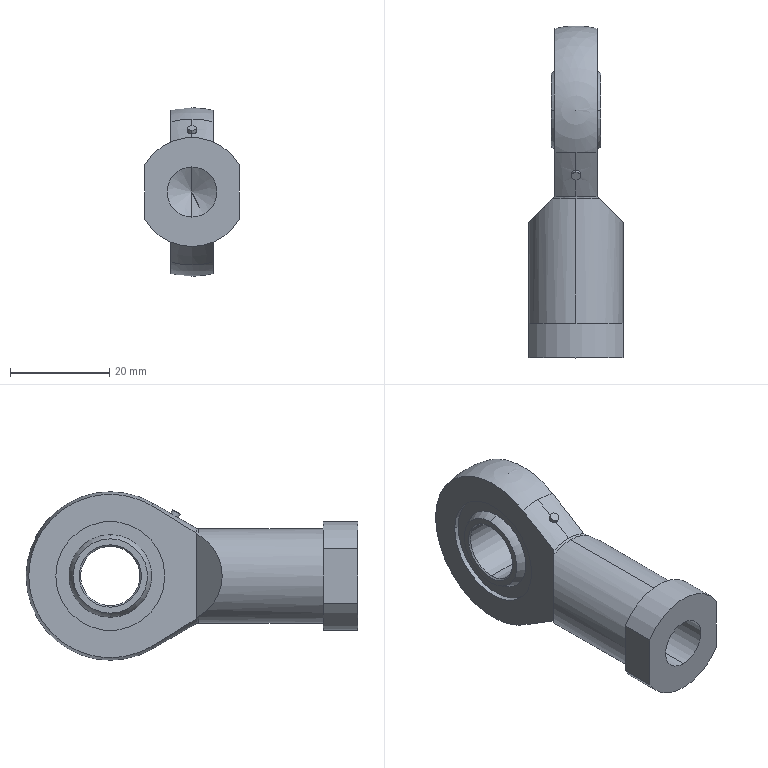Part | SolidWorks | features Revolution 3, ICE 2, RevCut 1 | 1 solid | 47 faces | box 19 x 67 x 34 mm | volume 14399 mm3 | cylinder 15 | plane 14 | cone 9 | torus 7 | sphere 2 | commonest cylinder face diameters 22 x7 1.788 x2 10.106 x2 12 x2 19 x2
STEP:
#1=CARTESIAN_POINT('',(0.,-12.56,13.366));
#2=VERTEX_POINT('',#1);
#3=CARTESIAN_POINT('',(0.,-14.11,12.474));
#4=VERTEX_POINT('',#3);
#5=CARTESIAN_POINT('',(0.,-13.335,12.92));
#6=DIRECTION('',(0.,0.4989,-0.8667));
#7=DIRECTION('',(0.,0.8667,0.4989));
#8=AXIS2_PLACEMENT_3D('',#5,#6,#7);
#9=CIRCLE('',#8,0.8942);
#10=EDGE_CURVE('',#2,#4,#9,.T.);
#11=ORIENTED_EDGE('',*,*,#10,.T.);
#12=CARTESIAN_POINT('',(0.,-13.686,11.737));
#13=VERTEX_POINT('',#12);
#14=CARTESIAN_POINT('',(0.,-13.686,11.737));
#15=DIRECTION('',(0.,0.4989,-0.8667));
#16=VECTOR('',#15,1000.);
#17=LINE('',#14,#16);
#18=EDGE_CURVE('',#4,#13,#17,.T.);
#19=ORIENTED_EDGE('',*,*,#18,.T.);
#20=CARTESIAN_POINT('',(0.,-12.136,12.63));
#21=VERTEX_POINT('',#20);
#22=CARTESIAN_POINT('',(0.,-13.686,11.737));
#23=CARTESIAN_POINT('',(0.1177,-13.686,11.737));
#24=CARTESIAN_POINT('',(0.2343,-13.665,11.748));
#25=CARTESIAN_POINT('',(0.4504,-13.585,11.788));
#26=CARTESIAN_POINT('',(0.5499,-13.525,11.817));
#27=CARTESIAN_POINT('',(0.7147,-13.378,11.893));
#28=CARTESIAN_POINT('',(0.7814,-13.29,11.94));
#29=CARTESIAN_POINT('',(0.8707,-13.101,12.043));
#30=CARTESIAN_POINT('',(0.8942,-12.998,12.1));
#31=CARTESIAN_POINT('',(0.8943,-12.796,12.217));
#32=CARTESIAN_POINT('',(0.8712,-12.696,12.277));
#33=CARTESIAN_POINT('',(0.7813,-12.51,12.39));
#34=CARTESIAN_POINT('',(0.7156,-12.426,12.442));
#35=CARTESIAN_POINT('',(0.5491,-12.286,12.532));
#36=CARTESIAN_POINT('',(0.4502,-12.23,12.568));
#37=CARTESIAN_POINT('',(0.2341,-12.155,12.617));
#38=CARTESIAN_POINT('',(0.1166,-12.136,12.63));
#39=CARTESIAN_POINT('',(0.,-12.136,12.63));
#40=B_SPLINE_CURVE_WITH_KNOTS('',3,(#22,#23,#24,#25,#26,#27,#28,#29,#30,#31,#32,#33,#34,#35,#36,#37,#38,#39),.UNSPECIFIED.,.F.,.F.,(4,2,2,2,2,2,2,2,4),(0.0003219,0.0006715,0.001021,0.001371,0.00172,0.00207,0.002419,0.002769,0.003119),.UNSPECIFIED.);
#41=EDGE_CURVE('',#13,#21,#40,.T.);
#42=ORIENTED_EDGE('',*,*,#41,.T.);
#43=CARTESIAN_POINT('',(0.,-12.136,12.63));
#44=DIRECTION('',(0.,0.4989,-0.8667));
#45=VECTOR('',#44,1000.);
#46=LINE('',#43,#45);
#47=EDGE_CURVE('',#2,#21,#46,.T.);
#48=ORIENTED_EDGE('',*,*,#47,.F.);
#49=EDGE_LOOP('',(#11,#19,#42,#48));
#50=FACE_OUTER_BOUND('',#49,.T.);
#51=CARTESIAN_POINT('',(0.,-12.911,12.183));
#52=DIRECTION('',(0.,0.4989,-0.8667));
#53=DIRECTION('',(0.,0.8667,0.4989));
#54=AXIS2_PLACEMENT_3D('',#51,#52,#53);
#55=CYLINDRICAL_SURFACE('',#54,0.8942);
#56=ADVANCED_FACE('',(#50),#55,.T.);
#57=CARTESIAN_POINT('',(5.,0.,7.5));
#58=VERTEX_POINT('',#57);
#59=CARTESIAN_POINT('',(5.,0.,-7.5));
#60=VERTEX_POINT('',#59);
#61=CARTESIAN_POINT('',(5.,0.,0.));
#62=DIRECTION('',(-1.,0.,0.));
#63=DIRECTION('',(0.,0.,1.));
#64=AXIS2_PLACEMENT_3D('',#61,#62,#63);
#65=CIRCLE('',#64,7.5);
#66=EDGE_CURVE('',#58,#60,#65,.T.);
#67=ORIENTED_EDGE('',*,*,#66,.T.);
#68=CARTESIAN_POINT('',(3.272,0.,-8.353));
#69=VERTEX_POINT('',#68);
#70=CARTESIAN_POINT('',(0.,0.,0.4455));
#71=DIRECTION('',(0.,1.,0.));
#72=DIRECTION('',(0.,0.,1.));
#73=AXIS2_PLACEMENT_3D('',#70,#71,#72);
#74=CIRCLE('',#73,9.388);
#75=EDGE_CURVE('',#60,#69,#74,.T.);
#76=ORIENTED_EDGE('',*,*,#75,.T.);
#77=CARTESIAN_POINT('',(3.272,0.,8.353));
#78=VERTEX_POINT('',#77);
#79=CARTESIAN_POINT('',(3.272,0.,0.));
#80=DIRECTION('',(-1.,0.,0.));
#81=DIRECTION('',(0.,0.,1.));
#82=AXIS2_PLACEMENT_3D('',#79,#80,#81);
#83=CIRCLE('',#82,8.353);
#84=EDGE_CURVE('',#78,#69,#83,.T.);
#85=ORIENTED_EDGE('',*,*,#84,.F.);
#86=CARTESIAN_POINT('',(0.,0.,-0.4455));
#87=DIRECTION('',(0.,-1.,0.));
#88=DIRECTION('',(0.,0.,-1.));
#89=AXIS2_PLACEMENT_3D('',#86,#87,#88);
#90=CIRCLE('',#89,9.388);
#91=EDGE_CURVE('',#58,#78,#90,.T.);
#92=ORIENTED_EDGE('',*,*,#91,.F.);
#93=EDGE_LOOP('',(#67,#76,#85,#92));
#94=FACE_OUTER_BOUND('',#93,.T.);
#95=CARTESIAN_POINT('',(0.,0.,0.));
#96=DIRECTION('',(-1.,0.,0.));
#97=DIRECTION('',(0.,0.,1.));
#98=AXIS2_PLACEMENT_3D('',#95,#96,#97);
#99=TOROIDAL_SURFACE('',#98,-0.4455,9.388);
#100=ADVANCED_FACE('',(#94),#99,.T.);
#101=CARTESIAN_POINT('',(4.7,0.,-6.));
#102=VERTEX_POINT('',#101);
#103=CARTESIAN_POINT('',(4.7,0.,6.));
#104=VERTEX_POINT('',#103);
#105=CARTESIAN_POINT('',(4.7,0.,0.));
#106=DIRECTION('',(-1.,0.,0.));
#107=DIRECTION('',(0.,0.,1.));
#108=AXIS2_PLACEMENT_3D('',#105,#106,#107);
#109=CIRCLE('',#108,6.);
#110=EDGE_CURVE('',#102,#104,#109,.T.);
#111=ORIENTED_EDGE('',*,*,#110,.T.);
#112=CARTESIAN_POINT('',(5.,0.,6.3));
#113=VERTEX_POINT('',#112);
#114=CARTESIAN_POINT('',(4.7,0.,6.));
#115=DIRECTION('',(0.7071,0.,0.7071));
#116=VECTOR('',#115,1000.);
#117=LINE('',#114,#116);
#118=EDGE_CURVE('',#104,#113,#117,.T.);
#119=ORIENTED_EDGE('',*,*,#118,.T.);
#120=CARTESIAN_POINT('',(5.,0.,-6.3));
#121=VERTEX_POINT('',#120);
#122=CARTESIAN_POINT('',(5.,0.,0.));
#123=DIRECTION('',(-1.,0.,0.));
#124=DIRECTION('',(0.,0.,1.));
#125=AXIS2_PLACEMENT_3D('',#122,#123,#124);
#126=CIRCLE('',#125,6.3);
#127=EDGE_CURVE('',#121,#113,#126,.T.);
#128=ORIENTED_EDGE('',*,*,#127,.F.);
#129=CARTESIAN_POINT('',(4.7,0.,-6.));
#130=DIRECTION('',(0.7071,0.,-0.7071));
#131=VECTOR('',#130,1000.);
#132=LINE('',#129,#131);
#133=EDGE_CURVE('',#102,#121,#132,.T.);
#134=ORIENTED_EDGE('',*,*,#133,.F.);
#135=EDGE_LOOP('',(#111,#119,#128,#134));
#136=FACE_OUTER_BOUND('',#135,.T.);
#137=CARTESIAN_POINT('',(4.7,0.,0.));
#138=DIRECTION('',(1.,0.,0.));
#139=DIRECTION('',(0.,0.,-1.));
#140=AXIS2_PLACEMENT_3D('',#137,#138,#139);
#141=CONICAL_SURFACE('',#140,6.,0.7854);
#142=ADVANCED_FACE('',(#136),#141,.F.);
#143=ORIENTED_EDGE('',*,*,#110,.F.);
#144=CARTESIAN_POINT('',(-4.7,0.,-6.));
#145=VERTEX_POINT('',#144);
#146=CARTESIAN_POINT('',(-5.,0.,-6.));
#147=DIRECTION('',(-1.,0.,0.));
#148=VECTOR('',#147,1000.);
#149=LINE('',#146,#148);
#150=EDGE_CURVE('',#102,#145,#149,.T.);
#151=ORIENTED_EDGE('',*,*,#150,.T.);
#152=CARTESIAN_POINT('',(-4.7,0.,6.));
#153=VERTEX_POINT('',#152);
#154=CARTESIAN_POINT('',(-4.7,0.,0.));
#155=DIRECTION('',(-1.,0.,0.));
#156=DIRECTION('',(0.,0.,1.));
#157=AXIS2_PLACEMENT_3D('',#154,#155,#156);
#158=CIRCLE('',#157,6.);
#159=EDGE_CURVE('',#145,#153,#158,.T.);
#160=ORIENTED_EDGE('',*,*,#159,.T.);
#161=CARTESIAN_POINT('',(-5.,0.,6.));
#162=DIRECTION('',(-1.,0.,0.));
#163=VECTOR('',#162,1000.);
#164=LINE('',#161,#163);
#165=EDGE_CURVE('',#104,#153,#164,.T.);
#166=ORIENTED_EDGE('',*,*,#165,.F.);
#167=EDGE_LOOP('',(#143,#151,#160,#166));
#168=FACE_OUTER_BOUND('',#167,.T.);
#169=CARTESIAN_POINT('',(-5.,0.,0.));
#170=DIRECTION('',(-1.,0.,0.));
#171=DIRECTION('',(0.,0.,1.));
#172=AXIS2_PLACEMENT_3D('',#169,#170,#171);
#173=CYLINDRICAL_SURFACE('',#172,6.);
#174=ADVANCED_FACE('',(#168),#173,.F.);
#175=ORIENTED_EDGE('',*,*,#159,.F.);
#176=CARTESIAN_POINT('',(-5.,0.,-6.3));
#177=VERTEX_POINT('',#176);
#178=CARTESIAN_POINT('',(-5.,0.,-6.3));
#179=DIRECTION('',(-0.7071,0.,-0.7071));
#180=VECTOR('',#179,1000.);
#181=LINE('',#178,#180);
#182=EDGE_CURVE('',#145,#177,#181,.T.);
#183=ORIENTED_EDGE('',*,*,#182,.T.);
#184=CARTESIAN_POINT('',(-5.,0.,6.3));
#185=VERTEX_POINT('',#184);
#186=CARTESIAN_POINT('',(-5.,0.,0.));
#187=DIRECTION('',(-1.,0.,0.));
#188=DIRECTION('',(0.,0.,1.));
#189=AXIS2_PLACEMENT_3D('',#186,#187,#188);
#190=CIRCLE('',#189,6.3);
#191=EDGE_CURVE('',#177,#185,#190,.T.);
#192=ORIENTED_EDGE('',*,*,#191,.T.);
#193=CARTESIAN_POINT('',(-5.,0.,6.3));
#194=DIRECTION('',(-0.7071,0.,0.7071));
#195=VECTOR('',#194,1000.);
#196=LINE('',#193,#195);
#197=EDGE_CURVE('',#153,#185,#196,.T.);
#198=ORIENTED_EDGE('',*,*,#197,.F.);
#199=EDGE_LOOP('',(#175,#183,#192,#198));
#200=FACE_OUTER_BOUND('',#199,.T.);
#201=CARTESIAN_POINT('',(-5.,0.,0.));
#202=DIRECTION('',(-1.,0.,0.));
#203=DIRECTION('',(0.,0.,1.));
#204=AXIS2_PLACEMENT_3D('',#201,#202,#203);
#205=CONICAL_SURFACE('',#204,6.3,0.7854);
#206=ADVANCED_FACE('',(#200),#205,.F.);
#207=CARTESIAN_POINT('',(-3.272,0.,8.353));
#208=VERTEX_POINT('',#207);
#209=CARTESIAN_POINT('',(-3.272,0.,-8.353));
#210=VERTEX_POINT('',#209);
#211=CARTESIAN_POINT('',(-3.272,0.,0.));
#212=DIRECTION('',(-1.,0.,0.));
#213=DIRECTION('',(0.,0.,1.));
#214=AXIS2_PLACEMENT_3D('',#211,#212,#213);
#215=CIRCLE('',#214,8.353);
#216=EDGE_CURVE('',#208,#210,#215,.T.);
#217=ORIENTED_EDGE('',*,*,#216,.T.);
#218=CARTESIAN_POINT('',(-5.,0.,-7.5));
#219=VERTEX_POINT('',#218);
#220=CARTESIAN_POINT('',(0.,0.,0.4455));
#221=DIRECTION('',(0.,1.,0.));
#222=DIRECTION('',(0.,0.,1.));
#223=AXIS2_PLACEMENT_3D('',#220,#221,#222);
#224=CIRCLE('',#223,9.388);
#225=EDGE_CURVE('',#210,#219,#224,.T.);
#226=ORIENTED_EDGE('',*,*,#225,.T.);
#227=CARTESIAN_POINT('',(-5.,0.,7.5));
#228=VERTEX_POINT('',#227);
#229=CARTESIAN_POINT('',(-5.,0.,0.));
#230=DIRECTION('',(-1.,0.,0.));
#231=DIRECTION('',(0.,0.,1.));
#232=AXIS2_PLACEMENT_3D('',#229,#230,#231);
#233=CIRCLE('',#232,7.5);
#234=EDGE_CURVE('',#228,#219,#233,.T.);
#235=ORIENTED_EDGE('',*,*,#234,.F.);
#236=CARTESIAN_POINT('',(0.,0.,-0.4455));
#237=DIRECTION('',(0.,-1.,0.));
#238=DIRECTION('',(0.,0.,-1.));
#239=AXIS2_PLACEMENT_3D('',#236,#237,#238);
#240=CIRCLE('',#239,9.388);
#241=EDGE_CURVE('',#208,#228,#240,.T.);
#242=ORIENTED_EDGE('',*,*,#241,.F.);
#243=EDGE_LOOP('',(#217,#226,#235,#242));
#244=FACE_OUTER_BOUND('',#243,.T.);
#245=CARTESIAN_POINT('',(0.,0.,0.));
#246=DIRECTION('',(-1.,0.,0.));
#247=DIRECTION('',(0.,0.,1.));
#248=AXIS2_PLACEMENT_3D('',#245,#246,#247);
#249=TOROIDAL_SURFACE('',#248,-0.4455,9.388);
#250=ADVANCED_FACE('',(#244),#249,.T.);
#251=CARTESIAN_POINT('',(0.,-25.483,0.));
#252=VERTEX_POINT('',#251);
#253=CARTESIAN_POINT('',(0.,-28.4,-5.053));
#254=VERTEX_POINT('',#253);
#255=CARTESIAN_POINT('',(0.,-26.219,-1.275));
#256=DIRECTION('',(0.,-0.5,-0.866));
#257=VECTOR('',#256,1000.);
#258=LINE('',#255,#257);
#259=EDGE_CURVE('',#252,#254,#258,.T.);
#260=ORIENTED_EDGE('',*,*,#259,.F.);
#261=CARTESIAN_POINT('',(0.,-28.4,5.053));
#262=VERTEX_POINT('',#261);
#263=CARTESIAN_POINT('',(0.,-26.219,1.275));
#264=DIRECTION('',(0.,-0.5,0.866));
#265=VECTOR('',#264,1000.);
#266=LINE('',#263,#265);
#267=EDGE_CURVE('',#252,#262,#266,.T.);
#268=ORIENTED_EDGE('',*,*,#267,.T.);
#269=CARTESIAN_POINT('',(0.,-28.4,0.));
#270=DIRECTION('',(0.,1.,0.));
#271=DIRECTION('',(0.,0.,1.));
#272=AXIS2_PLACEMENT_3D('',#269,#270,#271);
#273=CIRCLE('',#272,5.053);
#274=EDGE_CURVE('',#254,#262,#273,.T.);
#275=ORIENTED_EDGE('',*,*,#274,.F.);
#276=EDGE_LOOP('',(#260,#268,#275));
#277=FACE_OUTER_BOUND('',#276,.T.);
#278=CARTESIAN_POINT('',(0.,-26.219,0.));
#279=DIRECTION('',(0.,-1.,0.));
#280=DIRECTION('',(0.,0.,-1.));
#281=AXIS2_PLACEMENT_3D('',#278,#279,#280);
#282=CONICAL_SURFACE('',#281,1.275,1.047);
#283=ADVANCED_FACE('',(#277),#282,.F.);
#284=CARTESIAN_POINT('',(0.,-50.,-5.053));
#285=VERTEX_POINT('',#284);
#286=CARTESIAN_POINT('',(0.,-50.,5.053));
#287=VERTEX_POINT('',#286);
#288=CARTESIAN_POINT('',(0.,-50.,0.));
#289=DIRECTION('',(0.,1.,0.));
#290=DIRECTION('',(0.,0.,1.));
#291=AXIS2_PLACEMENT_3D('',#288,#289,#290);
#292=CIRCLE('',#291,5.053);
#293=EDGE_CURVE('',#285,#287,#292,.T.);
#294=ORIENTED_EDGE('',*,*,#293,.F.);
#295=CARTESIAN_POINT('',(0.,0.,-5.053));
#296=DIRECTION('',(0.,1.,0.));
#297=VECTOR('',#296,1000.);
#298=LINE('',#295,#297);
#299=EDGE_CURVE('',#285,#254,#298,.T.);
#300=ORIENTED_EDGE('',*,*,#299,.T.);
#301=ORIENTED_EDGE('',*,*,#274,.T.);
#302=CARTESIAN_POINT('',(0.,0.,5.053));
#303=DIRECTION('',(0.,1.,0.));
#304=VECTOR('',#303,1000.);
#305=LINE('',#302,#304);
#306=EDGE_CURVE('',#287,#262,#305,.T.);
#307=ORIENTED_EDGE('',*,*,#306,.F.);
#308=EDGE_LOOP('',(#294,#300,#301,#307));
#309=FACE_OUTER_BOUND('',#308,.T.);
#310=CARTESIAN_POINT('',(0.,0.,0.));
#311=DIRECTION('',(0.,1.,0.));
#312=DIRECTION('',(0.,0.,1.));
#313=AXIS2_PLACEMENT_3D('',#310,#311,#312);
#314=CYLINDRICAL_SURFACE('',#313,5.053);
#315=ADVANCED_FACE('',(#309),#314,.F.);
#316=CARTESIAN_POINT('',(0.,-17.84,-9.5));
#317=VERTEX_POINT('',#316);
#318=CARTESIAN_POINT('',(4.749,-17.84,-8.228));
#319=VERTEX_POINT('',#318);
#320=CARTESIAN_POINT('',(0.,-17.84,0.));
#321=DIRECTION('',(0.,-1.,0.));
#322=DIRECTION('',(0.,0.,-1.));
#323=AXIS2_PLACEMENT_3D('',#320,#321,#322);
#324=CIRCLE('',#323,9.5);
#325=EDGE_CURVE('',#317,#319,#324,.T.);
#326=ORIENTED_EDGE('',*,*,#325,.F.);
#327=CARTESIAN_POINT('',(0.,-17.341,-9.633));
#328=VERTEX_POINT('',#327);
#329=CARTESIAN_POINT('',(0.,-17.84,-10.5));
#330=DIRECTION('',(-1.,0.,0.));
#331=DIRECTION('',(0.,0.,1.));
#332=AXIS2_PLACEMENT_3D('',#329,#330,#331);
#333=CIRCLE('',#332,1.);
#334=EDGE_CURVE('',#317,#328,#333,.T.);
#335=ORIENTED_EDGE('',*,*,#334,.T.);
#336=CARTESIAN_POINT('',(4.25,-17.341,-8.645));
#337=VERTEX_POINT('',#336);
#338=CARTESIAN_POINT('',(0.,-17.341,0.));
#339=DIRECTION('',(0.,-1.,0.));
#340=DIRECTION('',(0.,0.,-1.));
#341=AXIS2_PLACEMENT_3D('',#338,#339,#340);
#342=CIRCLE('',#341,9.633);
#343=EDGE_CURVE('',#328,#337,#342,.T.);
#344=ORIENTED_EDGE('',*,*,#343,.T.);
#345=CARTESIAN_POINT('',(4.749,-17.84,-8.228));
#346=CARTESIAN_POINT('',(4.568,-17.659,-8.332));
#347=CARTESIAN_POINT('',(4.402,-17.493,-8.473));
#348=CARTESIAN_POINT('',(4.25,-17.341,-8.645));
#349=B_SPLINE_CURVE_WITH_KNOTS('',3,(#345,#346,#347,#348),.UNSPECIFIED.,.F.,.F.,(4,4),(0.000000302,0.00082),.UNSPECIFIED.);
#350=EDGE_CURVE('',#319,#337,#349,.T.);
#351=ORIENTED_EDGE('',*,*,#350,.F.);
#352=EDGE_LOOP('',(#326,#335,#344,#351));
#353=FACE_OUTER_BOUND('',#352,.T.);
#354=CARTESIAN_POINT('',(0.,-17.84,0.));
#355=DIRECTION('',(0.,-1.,0.));
#356=DIRECTION('',(0.,0.,-1.));
#357=AXIS2_PLACEMENT_3D('',#354,#355,#356);
#358=TOROIDAL_SURFACE('',#357,10.5,1.);
#359=ADVANCED_FACE('',(#353),#358,.F.);
#360=CARTESIAN_POINT('',(4.749,-17.84,8.228));
#361=VERTEX_POINT('',#360);
#362=CARTESIAN_POINT('',(0.,-17.84,9.5));
#363=VERTEX_POINT('',#362);
#364=CARTESIAN_POINT('',(0.,-17.84,0.));
#365=DIRECTION('',(0.,-1.,0.));
#366=DIRECTION('',(0.,0.,-1.));
#367=AXIS2_PLACEMENT_3D('',#364,#365,#366);
#368=CIRCLE('',#367,9.5);
#369=EDGE_CURVE('',#361,#363,#368,.T.);
#370=ORIENTED_EDGE('',*,*,#369,.T.);
#371=CARTESIAN_POINT('',(0.,-43.,9.5));
#372=VERTEX_POINT('',#371);
#373=CARTESIAN_POINT('',(0.,-50.,9.5));
#374=DIRECTION('',(0.,-1.,0.));
#375=VECTOR('',#374,1000.);
#376=LINE('',#373,#375);
#377=EDGE_CURVE('',#363,#372,#376,.T.);
#378=ORIENTED_EDGE('',*,*,#377,.T.);
#379=CARTESIAN_POINT('',(9.5,-43.,0.));
#380=VERTEX_POINT('',#379);
#381=CARTESIAN_POINT('',(0.,-43.,0.));
#382=DIRECTION('',(0.,-1.,0.));
#383=DIRECTION('',(0.,0.,-1.));
#384=AXIS2_PLACEMENT_3D('',#381,#382,#383);
#385=CIRCLE('',#384,9.5);
#386=EDGE_CURVE('',#380,#372,#385,.T.);
#387=ORIENTED_EDGE('',*,*,#386,.F.);
#388=CARTESIAN_POINT('',(0.,-43.,-9.5));
#389=VERTEX_POINT('',#388);
#390=CARTESIAN_POINT('',(0.,-43.,0.));
#391=DIRECTION('',(0.,-1.,0.));
#392=DIRECTION('',(0.,0.,-1.));
#393=AXIS2_PLACEMENT_3D('',#390,#391,#392);
#394=CIRCLE('',#393,9.5);
#395=EDGE_CURVE('',#389,#380,#394,.T.);
#396=ORIENTED_EDGE('',*,*,#395,.F.);
#397=CARTESIAN_POINT('',(0.,-50.,-9.5));
#398=DIRECTION('',(0.,-1.,0.));
#399=VECTOR('',#398,1000.);
#400=LINE('',#397,#399);
#401=EDGE_CURVE('',#317,#389,#400,.T.);
#402=ORIENTED_EDGE('',*,*,#401,.F.);
#403=ORIENTED_EDGE('',*,*,#325,.T.);
#404=CARTESIAN_POINT('',(4.749,-17.84,8.228));
#405=CARTESIAN_POINT('',(11.876,-24.967,4.114));
#406=CARTESIAN_POINT('',(11.876,-24.967,-4.114));
#407=CARTESIAN_POINT('',(4.749,-17.84,-8.228));
#408=(BOUNDED_CURVE()B_SPLINE_CURVE(3,(#404,#405,#406,#407),.UNSPECIFIED.,.F.,.T.)B_SPLINE_CURVE_WITH_KNOTS((4,4),(5.236,7.331),.UNSPECIFIED.)CURVE()GEOMETRIC_REPRESENTATION_ITEM()RATIONAL_B_SPLINE_CURVE((1.,0.6666,0.6666,1.))REPRESENTATION_ITEM(''));
#409=EDGE_CURVE('',#361,#319,#408,.T.);
#410=ORIENTED_EDGE('',*,*,#409,.F.);
#411=EDGE_LOOP('',(#370,#378,#387,#396,#402,#403,#410));
#412=FACE_OUTER_BOUND('',#411,.T.);
#413=CARTESIAN_POINT('',(0.,-50.,0.));
#414=DIRECTION('',(0.,-1.,0.));
#415=DIRECTION('',(0.,0.,-1.));
#416=AXIS2_PLACEMENT_3D('',#413,#414,#415);
#417=CYLINDRICAL_SURFACE('',#416,9.5);
#418=ADVANCED_FACE('',(#412),#417,.T.);
#419=CARTESIAN_POINT('',(0.,17.,0.));
#420=VERTEX_POINT('',#419);
#421=CARTESIAN_POINT('',(4.25,16.46,0.));
#422=VERTEX_POINT('',#421);
#423=CARTESIAN_POINT('',(0.,0.,0.));
#424=DIRECTION('',(0.,0.,-1.));
#425=DIRECTION('',(-1.,0.,0.));
#426=AXIS2_PLACEMENT_3D('',#423,#424,#425);
#427=CIRCLE('',#426,17.);
#428=EDGE_CURVE('',#420,#422,#427,.T.);
#429=ORIENTED_EDGE('',*,*,#428,.F.);
#430=CARTESIAN_POINT('',(-4.25,16.46,0.));
#431=VERTEX_POINT('',#430);
#432=CARTESIAN_POINT('',(0.,0.,0.));
#433=DIRECTION('',(0.,0.,1.));
#434=DIRECTION('',(1.,0.,0.));
#435=AXIS2_PLACEMENT_3D('',#432,#433,#434);
#436=CIRCLE('',#435,17.);
#437=EDGE_CURVE('',#420,#431,#436,.T.);
#438=ORIENTED_EDGE('',*,*,#437,.T.);
#439=CARTESIAN_POINT('',(-4.25,-8.481,14.107));
#440=VERTEX_POINT('',#439);
#441=CARTESIAN_POINT('',(-4.25,0.,0.));
#442=DIRECTION('',(-1.,0.,0.));
#443=DIRECTION('',(0.,1.,0.));
#444=AXIS2_PLACEMENT_3D('',#441,#442,#443);
#445=CIRCLE('',#444,16.46);
#446=EDGE_CURVE('',#440,#431,#445,.T.);
#447=ORIENTED_EDGE('',*,*,#446,.F.);
#448=CARTESIAN_POINT('',(0.,-8.481,14.733));
#449=VERTEX_POINT('',#448);
#450=CARTESIAN_POINT('',(0.,-8.481,0.));
#451=DIRECTION('',(0.,-1.,0.));
#452=DIRECTION('',(0.,0.,-1.));
#453=AXIS2_PLACEMENT_3D('',#450,#451,#452);
#454=CIRCLE('',#453,14.733);
#455=EDGE_CURVE('',#449,#440,#454,.T.);
#456=ORIENTED_EDGE('',*,*,#455,.F.);
#457=CARTESIAN_POINT('',(4.25,-8.481,14.107));
#458=VERTEX_POINT('',#457);
#459=CARTESIAN_POINT('',(0.,-8.481,0.));
#460=DIRECTION('',(0.,-1.,0.));
#461=DIRECTION('',(0.,0.,-1.));
#462=AXIS2_PLACEMENT_3D('',#459,#460,#461);
#463=CIRCLE('',#462,14.733);
#464=EDGE_CURVE('',#458,#449,#463,.T.);
#465=ORIENTED_EDGE('',*,*,#464,.F.);
#466=CARTESIAN_POINT('',(4.25,0.,0.));
#467=DIRECTION('',(1.,0.,0.));
#468=DIRECTION('',(0.,-1.,0.));
#469=AXIS2_PLACEMENT_3D('',#466,#467,#468);
#470=CIRCLE('',#469,16.46);
#471=EDGE_CURVE('',#422,#458,#470,.T.);
#472=ORIENTED_EDGE('',*,*,#471,.F.);
#473=EDGE_LOOP('',(#429,#438,#447,#456,#465,#472));
#474=FACE_OUTER_BOUND('',#473,.T.);
#475=CARTESIAN_POINT('',(0.,0.,0.));
#476=DIRECTION('',(0.,0.,1.));
#477=DIRECTION('',(1.,0.,0.));
#478=AXIS2_PLACEMENT_3D('',#475,#476,#477);
#479=SPHERICAL_SURFACE('',#478,17.);
#480=ADVANCED_FACE('',(#474),#479,.T.);
#481=CARTESIAN_POINT('',(0.,-17.341,9.633));
#482=VERTEX_POINT('',#481);
#483=CARTESIAN_POINT('',(-4.25,-17.341,8.645));
#484=VERTEX_POINT('',#483);
#485=CARTESIAN_POINT('',(0.,-17.341,0.));
#486=DIRECTION('',(0.,-1.,0.));
#487=DIRECTION('',(0.,0.,-1.));
#488=AXIS2_PLACEMENT_3D('',#485,#486,#487);
#489=CIRCLE('',#488,9.633);
#490=EDGE_CURVE('',#482,#484,#489,.T.);
#491=ORIENTED_EDGE('',*,*,#490,.F.);
#492=CARTESIAN_POINT('',(0.,-17.341,9.633));
#493=DIRECTION('',(0.,0.8667,0.4989));
#494=VECTOR('',#493,1000.);
#495=LINE('',#492,#494);
#496=EDGE_CURVE('',#482,#13,#495,.T.);
#497=ORIENTED_EDGE('',*,*,#496,.T.);
#498=CARTESIAN_POINT('',(0.,-12.136,12.63));
#499=CARTESIAN_POINT('',(-0.1166,-12.136,12.63));
#500=CARTESIAN_POINT('',(-0.2343,-12.156,12.617));
#501=CARTESIAN_POINT('',(-0.4496,-12.23,12.568));
#502=CARTESIAN_POINT('',(-0.5492,-12.286,12.531));
#503=CARTESIAN_POINT('',(-0.7145,-12.425,12.443));
#504=CARTESIAN_POINT('',(-0.7808,-12.509,12.39));
#505=CARTESIAN_POINT('',(-0.8709,-12.694,12.277));
#506=CARTESIAN_POINT('',(-0.8942,-12.794,12.218));
#507=CARTESIAN_POINT('',(-0.8943,-12.998,12.1));
#508=CARTESIAN_POINT('',(-0.8711,-13.1,12.043));
#509=CARTESIAN_POINT('',(-0.7816,-13.29,11.94));
#510=CARTESIAN_POINT('',(-0.7152,-13.378,11.893));
#511=CARTESIAN_POINT('',(-0.5506,-13.525,11.818));
#512=CARTESIAN_POINT('',(-0.4513,-13.584,11.788));
#513=CARTESIAN_POINT('',(-0.2337,-13.665,11.747));
#514=CARTESIAN_POINT('',(-0.1177,-13.686,11.737));
#515=CARTESIAN_POINT('',(0.,-13.686,11.737));
#516=B_SPLINE_CURVE_WITH_KNOTS('',3,(#498,#499,#500,#501,#502,#503,#504,#505,#506,#507,#508,#509,#510,#511,#512,#513,#514,#515),.UNSPECIFIED.,.F.,.F.,(4,2,2,2,2,2,2,2,4),(0.003119,0.003468,0.003818,0.004167,0.004517,0.004866,0.005215,0.005565,0.005914),.UNSPECIFIED.);
#517=EDGE_CURVE('',#21,#13,#516,.T.);
#518=ORIENTED_EDGE('',*,*,#517,.F.);
#519=CARTESIAN_POINT('',(0.,-17.341,9.633));
#520=DIRECTION('',(0.,0.8667,0.4989));
#521=VECTOR('',#520,1000.);
#522=LINE('',#519,#521);
#523=EDGE_CURVE('',#21,#449,#522,.T.);
#524=ORIENTED_EDGE('',*,*,#523,.T.);
#525=ORIENTED_EDGE('',*,*,#455,.T.);
#526=CARTESIAN_POINT('',(-4.25,-17.341,8.645));
#527=CARTESIAN_POINT('',(-4.25,-15.882,9.581));
#528=CARTESIAN_POINT('',(-4.25,-14.409,10.498));
#529=CARTESIAN_POINT('',(-4.25,-11.452,12.314));
#530=CARTESIAN_POINT('',(-4.25,-9.968,13.213));
#531=CARTESIAN_POINT('',(-4.25,-8.481,14.107));
#532=B_SPLINE_CURVE_WITH_KNOTS('',3,(#526,#527,#528,#529,#530,#531),.UNSPECIFIED.,.F.,.F.,(4,2,4),(0.05787,0.06306,0.06824),.UNSPECIFIED.);
#533=EDGE_CURVE('',#484,#440,#532,.T.);
#534=ORIENTED_EDGE('',*,*,#533,.F.);
#535=EDGE_LOOP('',(#491,#497,#518,#524,#525,#534));
#536=FACE_OUTER_BOUND('',#535,.T.);
#537=CARTESIAN_POINT('',(0.,-17.341,0.));
#538=DIRECTION('',(0.,1.,0.));
#539=DIRECTION('',(0.,0.,1.));
#540=AXIS2_PLACEMENT_3D('',#537,#538,#539);
#541=CONICAL_SURFACE('',#540,9.633,0.5223);
#542=ADVANCED_FACE('',(#536),#541,.T.);
#543=CARTESIAN_POINT('',(-9.5,-43.,-5.545));
#544=VERTEX_POINT('',#543);
#545=CARTESIAN_POINT('',(0.,-43.,-11.));
#546=VERTEX_POINT('',#545);
#547=CARTESIAN_POINT('',(0.,-43.,0.));
#548=DIRECTION('',(0.,-1.,0.));
#549=DIRECTION('',(0.,0.,-1.));
#550=AXIS2_PLACEMENT_3D('',#547,#548,#549);
#551=CIRCLE('',#550,11.);
#552=EDGE_CURVE('',#544,#546,#551,.T.);
#553=ORIENTED_EDGE('',*,*,#552,.T.);
#554=CARTESIAN_POINT('',(0.,-50.,-11.));
#555=VERTEX_POINT('',#554);
#556=CARTESIAN_POINT('',(0.,-50.,-11.));
#557=DIRECTION('',(0.,-1.,0.));
#558=VECTOR('',#557,1000.);
#559=LINE('',#556,#558);
#560=EDGE_CURVE('',#546,#555,#559,.T.);
#561=ORIENTED_EDGE('',*,*,#560,.T.);
#562=CARTESIAN_POINT('',(-9.5,-50.,-5.545));
#563=VERTEX_POINT('',#562);
#564=CARTESIAN_POINT('',(0.,-50.,0.));
#565=DIRECTION('',(0.,-1.,0.));
#566=DIRECTION('',(0.,0.,-1.));
#567=AXIS2_PLACEMENT_3D('',#564,#565,#566);
#568=CIRCLE('',#567,11.);
#569=EDGE_CURVE('',#563,#555,#568,.T.);
#570=ORIENTED_EDGE('',*,*,#569,.F.);
#571=CARTESIAN_POINT('',(-9.5,-50.,-5.545));
#572=DIRECTION('',(0.,-1.,0.));
#573=VECTOR('',#572,1000.);
#574=LINE('',#571,#573);
#575=EDGE_CURVE('',#544,#563,#574,.T.);
#576=ORIENTED_EDGE('',*,*,#575,.F.);
#577=EDGE_LOOP('',(#553,#561,#570,#576));
#578=FACE_OUTER_BOUND('',#577,.T.);
#579=CARTESIAN_POINT('',(0.,-50.,0.));
#580=DIRECTION('',(0.,-1.,0.));
#581=DIRECTION('',(0.,0.,-1.));
#582=AXIS2_PLACEMENT_3D('',#579,#580,#581);
#583=CYLINDRICAL_SURFACE('',#582,11.);
#584=ADVANCED_FACE('',(#578),#583,.T.);
#585=CARTESIAN_POINT('',(-4.25,11.,0.));
#586=VERTEX_POINT('',#585);
#587=CARTESIAN_POINT('',(-4.25,-11.,0.));
#588=VERTEX_POINT('',#587);
#589=CARTESIAN_POINT('',(-4.25,0.,0.));
#590=DIRECTION('',(-1.,0.,0.));
#591=DIRECTION('',(0.,1.,0.));
#592=AXIS2_PLACEMENT_3D('',#589,#590,#591);
#593=CIRCLE('',#592,11.);
#594=EDGE_CURVE('',#586,#588,#593,.T.);
#595=ORIENTED_EDGE('',*,*,#594,.T.);
#596=CARTESIAN_POINT('',(-3.272,-11.,0.));
#597=VERTEX_POINT('',#596);
#598=CARTESIAN_POINT('',(-9.5,-11.,0.));
#599=DIRECTION('',(1.,0.,0.));
#600=VECTOR('',#599,1000.);
#601=LINE('',#598,#600);
#602=EDGE_CURVE('',#588,#597,#601,.T.);
#603=ORIENTED_EDGE('',*,*,#602,.T.);
#604=CARTESIAN_POINT('',(-3.272,11.,0.));
#605=VERTEX_POINT('',#604);
#606=CARTESIAN_POINT('',(-3.272,0.,0.));
#607=DIRECTION('',(-1.,0.,0.));
#608=DIRECTION('',(0.,0.,1.));
#609=AXIS2_PLACEMENT_3D('',#606,#607,#608);
#610=CIRCLE('',#609,11.);
#611=EDGE_CURVE('',#605,#597,#610,.T.);
#612=ORIENTED_EDGE('',*,*,#611,.F.);
#613=CARTESIAN_POINT('',(-9.5,11.,0.));
#614=DIRECTION('',(1.,0.,0.));
#615=VECTOR('',#614,1000.);
#616=LINE('',#613,#615);
#617=EDGE_CURVE('',#586,#605,#616,.T.);
#618=ORIENTED_EDGE('',*,*,#617,.F.);
#619=EDGE_LOOP('',(#595,#603,#612,#618));
#620=FACE_OUTER_BOUND('',#619,.T.);
#621=CARTESIAN_POINT('',(-9.5,0.,0.));
#622=DIRECTION('',(1.,0.,0.));
#623=DIRECTION('',(0.,1.,0.));
#624=AXIS2_PLACEMENT_3D('',#621,#622,#623);
#625=CYLINDRICAL_SURFACE('',#624,11.);
#626=ADVANCED_FACE('',(#620),#625,.F.);
#627=CARTESIAN_POINT('',(3.272,11.,0.));
#628=VERTEX_POINT('',#627);
#629=CARTESIAN_POINT('',(3.272,-11.,0.));
#630=VERTEX_POINT('',#629);
#631=CARTESIAN_POINT('',(3.272,0.,0.));
#632=DIRECTION('',(-1.,0.,0.));
#633=DIRECTION('',(0.,0.,1.));
#634=AXIS2_PLACEMENT_3D('',#631,#632,#633);
#635=CIRCLE('',#634,11.);
#636=EDGE_CURVE('',#628,#630,#635,.T.);
#637=ORIENTED_EDGE('',*,*,#636,.T.);
#638=CARTESIAN_POINT('',(4.25,-11.,0.));
#639=VERTEX_POINT('',#638);
#640=CARTESIAN_POINT('',(-9.5,-11.,0.));
#641=DIRECTION('',(1.,0.,0.));
#642=VECTOR('',#641,1000.);
#643=LINE('',#640,#642);
#644=EDGE_CURVE('',#630,#639,#643,.T.);
#645=ORIENTED_EDGE('',*,*,#644,.T.);
#646=CARTESIAN_POINT('',(4.25,11.,0.));
#647=VERTEX_POINT('',#646);
#648=CARTESIAN_POINT('',(4.25,0.,0.));
#649=DIRECTION('',(-1.,0.,0.));
#650=DIRECTION('',(0.,-1.,0.));
#651=AXIS2_PLACEMENT_3D('',#648,#649,#650);
#652=CIRCLE('',#651,11.);
#653=EDGE_CURVE('',#647,#639,#652,.T.);
#654=ORIENTED_EDGE('',*,*,#653,.F.);
#655=CARTESIAN_POINT('',(-9.5,11.,0.));
#656=DIRECTION('',(1.,0.,0.));
#657=VECTOR('',#656,1000.);
#658=LINE('',#655,#657);
#659=EDGE_CURVE('',#628,#647,#658,.T.);
#660=ORIENTED_EDGE('',*,*,#659,.F.);
#661=EDGE_LOOP('',(#637,#645,#654,#660));
#662=FACE_OUTER_BOUND('',#661,.T.);
#663=CARTESIAN_POINT('',(-9.5,0.,0.));
#664=DIRECTION('',(1.,0.,0.));
#665=DIRECTION('',(0.,1.,0.));
#666=AXIS2_PLACEMENT_3D('',#663,#664,#665);
#667=CYLINDRICAL_SURFACE('',#666,11.);
#668=ADVANCED_FACE('',(#662),#667,.F.);
#669=ORIENTED_EDGE('',*,*,#644,.F.);
#670=CARTESIAN_POINT('',(3.272,0.,0.));
#671=DIRECTION('',(-1.,0.,0.));
#672=DIRECTION('',(0.,0.,1.));
#673=AXIS2_PLACEMENT_3D('',#670,#671,#672);
#674=CIRCLE('',#673,11.);
#675=EDGE_CURVE('',#630,#628,#674,.T.);
#676=ORIENTED_EDGE('',*,*,#675,.T.);
#677=ORIENTED_EDGE('',*,*,#659,.T.);
#678=CARTESIAN_POINT('',(4.25,0.,0.));
#679=DIRECTION('',(-1.,0.,0.));
#680=DIRECTION('',(0.,-1.,0.));
#681=AXIS2_PLACEMENT_3D('',#678,#679,#680);
#682=CIRCLE('',#681,11.);
#683=EDGE_CURVE('',#639,#647,#682,.T.);
#684=ORIENTED_EDGE('',*,*,#683,.F.);
#685=EDGE_LOOP('',(#669,#676,#677,#684));
#686=FACE_OUTER_BOUND('',#685,.T.);
#687=CARTESIAN_POINT('',(-9.5,0.,0.));
#688=DIRECTION('',(1.,0.,0.));
#689=DIRECTION('',(0.,1.,0.));
#690=AXIS2_PLACEMENT_3D('',#687,#688,#689);
#691=CYLINDRICAL_SURFACE('',#690,11.);
#692=ADVANCED_FACE('',(#686),#691,.F.);
#693=ORIENTED_EDGE('',*,*,#602,.F.);
#694=CARTESIAN_POINT('',(-4.25,0.,0.));
#695=DIRECTION('',(-1.,0.,0.));
#696=DIRECTION('',(0.,1.,0.));
#697=AXIS2_PLACEMENT_3D('',#694,#695,#696);
#698=CIRCLE('',#697,11.);
#699=EDGE_CURVE('',#588,#586,#698,.T.);
#700=ORIENTED_EDGE('',*,*,#699,.T.);
#701=ORIENTED_EDGE('',*,*,#617,.T.);
#702=CARTESIAN_POINT('',(-3.272,0.,0.));
#703=DIRECTION('',(-1.,0.,0.));
#704=DIRECTION('',(0.,0.,1.));
#705=AXIS2_PLACEMENT_3D('',#702,#703,#704);
#706=CIRCLE('',#705,11.);
#707=EDGE_CURVE('',#597,#605,#706,.T.);
#708=ORIENTED_EDGE('',*,*,#707,.F.);
#709=EDGE_LOOP('',(#693,#700,#701,#708));
#710=FACE_OUTER_BOUND('',#709,.T.);
#711=CARTESIAN_POINT('',(-9.5,0.,0.));
#712=DIRECTION('',(1.,0.,0.));
#713=DIRECTION('',(0.,1.,0.));
#714=AXIS2_PLACEMENT_3D('',#711,#712,#713);
#715=CYLINDRICAL_SURFACE('',#714,11.);
#716=ADVANCED_FACE('',(#710),#715,.F.);
#717=CARTESIAN_POINT('',(4.25,-17.341,8.645));
#718=VERTEX_POINT('',#717);
#719=CARTESIAN_POINT('',(4.25,-8.481,14.107));
#720=CARTESIAN_POINT('',(4.25,-9.968,13.213));
#721=CARTESIAN_POINT('',(4.25,-11.451,12.315));
#722=CARTESIAN_POINT('',(4.25,-14.408,10.499));
#723=CARTESIAN_POINT('',(4.25,-15.88,9.582));
#724=CARTESIAN_POINT('',(4.25,-17.341,8.645));
#725=B_SPLINE_CURVE_WITH_KNOTS('',3,(#719,#720,#721,#722,#723,#724),.UNSPECIFIED.,.F.,.F.,(4,2,4),(0.02144,0.02664,0.03184),.UNSPECIFIED.);
#726=EDGE_CURVE('',#458,#718,#725,.T.);
#727=ORIENTED_EDGE('',*,*,#726,.T.);
#728=CARTESIAN_POINT('',(4.25,-17.341,-17.));
#729=DIRECTION('',(0.,0.,1.));
#730=VECTOR('',#729,1000.);
#731=LINE('',#728,#730);
#732=EDGE_CURVE('',#337,#718,#731,.T.);
#733=ORIENTED_EDGE('',*,*,#732,.F.);
#734=CARTESIAN_POINT('',(4.25,-8.481,-14.107));
#735=VERTEX_POINT('',#734);
#736=CARTESIAN_POINT('',(4.25,-17.341,-8.645));
#737=CARTESIAN_POINT('',(4.25,-15.882,-9.581));
#738=CARTESIAN_POINT('',(4.25,-14.409,-10.498));
#739=CARTESIAN_POINT('',(4.25,-11.452,-12.314));
#740=CARTESIAN_POINT('',(4.25,-9.968,-13.213));
#741=CARTESIAN_POINT('',(4.25,-8.481,-14.107));
#742=B_SPLINE_CURVE_WITH_KNOTS('',3,(#736,#737,#738,#739,#740,#741),.UNSPECIFIED.,.F.,.F.,(4,2,4),(0.05787,0.06306,0.06824),.UNSPECIFIED.);
#743=EDGE_CURVE('',#337,#735,#742,.T.);
#744=ORIENTED_EDGE('',*,*,#743,.T.);
#745=CARTESIAN_POINT('',(4.25,0.,0.));
#746=DIRECTION('',(1.,0.,0.));
#747=DIRECTION('',(0.,-1.,0.));
#748=AXIS2_PLACEMENT_3D('',#745,#746,#747);
#749=CIRCLE('',#748,16.46);
#750=EDGE_CURVE('',#735,#422,#749,.T.);
#751=ORIENTED_EDGE('',*,*,#750,.T.);
#752=ORIENTED_EDGE('',*,*,#471,.T.);
#753=EDGE_LOOP('',(#727,#733,#744,#751,#752));
#754=FACE_OUTER_BOUND('',#753,.T.);
#755=ORIENTED_EDGE('',*,*,#653,.T.);
#756=ORIENTED_EDGE('',*,*,#683,.T.);
#757=EDGE_LOOP('',(#755,#756));
#758=FACE_BOUND('',#757,.T.);
#759=CARTESIAN_POINT('',(4.25,16.46,-17.));
#760=DIRECTION('',(-1.,0.,0.));
#761=DIRECTION('',(0.,-1.,0.));
#762=AXIS2_PLACEMENT_3D('',#759,#760,#761);
#763=PLANE('',#762);
#764=ADVANCED_FACE('',(#754,#758),#763,.F.);
#765=CARTESIAN_POINT('',(-4.25,-8.481,-14.107));
#766=VERTEX_POINT('',#765);
#767=CARTESIAN_POINT('',(-4.25,-17.341,-8.645));
#768=VERTEX_POINT('',#767);
#769=CARTESIAN_POINT('',(-4.25,-8.481,-14.107));
#770=CARTESIAN_POINT('',(-4.25,-9.968,-13.213));
#771=CARTESIAN_POINT('',(-4.25,-11.451,-12.315));
#772=CARTESIAN_POINT('',(-4.25,-14.408,-10.499));
#773=CARTESIAN_POINT('',(-4.25,-15.88,-9.582));
#774=CARTESIAN_POINT('',(-4.25,-17.341,-8.645));
#775=B_SPLINE_CURVE_WITH_KNOTS('',3,(#769,#770,#771,#772,#773,#774),.UNSPECIFIED.,.F.,.F.,(4,2,4),(0.02144,0.02664,0.03184),.UNSPECIFIED.);
#776=EDGE_CURVE('',#766,#768,#775,.T.);
#777=ORIENTED_EDGE('',*,*,#776,.T.);
#778=CARTESIAN_POINT('',(-4.25,-17.341,-17.));
#779=DIRECTION('',(0.,0.,1.));
#780=VECTOR('',#779,1000.);
#781=LINE('',#778,#780);
#782=EDGE_CURVE('',#768,#484,#781,.T.);
#783=ORIENTED_EDGE('',*,*,#782,.T.);
#784=ORIENTED_EDGE('',*,*,#533,.T.);
#785=ORIENTED_EDGE('',*,*,#446,.T.);
#786=CARTESIAN_POINT('',(-4.25,0.,0.));
#787=DIRECTION('',(-1.,0.,0.));
#788=DIRECTION('',(0.,1.,0.));
#789=AXIS2_PLACEMENT_3D('',#786,#787,#788);
#790=CIRCLE('',#789,16.46);
#791=EDGE_CURVE('',#431,#766,#790,.T.);
#792=ORIENTED_EDGE('',*,*,#791,.T.);
#793=EDGE_LOOP('',(#777,#783,#784,#785,#792));
#794=FACE_OUTER_BOUND('',#793,.T.);
#795=ORIENTED_EDGE('',*,*,#594,.F.);
#796=ORIENTED_EDGE('',*,*,#699,.F.);
#797=EDGE_LOOP('',(#795,#796));
#798=FACE_BOUND('',#797,.T.);
#799=CARTESIAN_POINT('',(-4.25,16.46,-17.));
#800=DIRECTION('',(1.,0.,0.));
#801=DIRECTION('',(0.,1.,0.));
#802=AXIS2_PLACEMENT_3D('',#799,#800,#801);
#803=PLANE('',#802);
#804=ADVANCED_FACE('',(#794,#798),#803,.F.);
#805=CARTESIAN_POINT('',(-9.5,-50.,5.545));
#806=VERTEX_POINT('',#805);
#807=CARTESIAN_POINT('',(-9.5,-50.,-17.));
#808=DIRECTION('',(0.,0.,1.));
#809=VECTOR('',#808,1000.);
#810=LINE('',#807,#809);
#811=EDGE_CURVE('',#563,#806,#810,.T.);
#812=ORIENTED_EDGE('',*,*,#811,.F.);
#813=ORIENTED_EDGE('',*,*,#569,.T.);
#814=CARTESIAN_POINT('',(9.5,-50.,-5.545));
#815=VERTEX_POINT('',#814);
#816=CARTESIAN_POINT('',(0.,-50.,0.));
#817=DIRECTION('',(0.,-1.,0.));
#818=DIRECTION('',(0.,0.,-1.));
#819=AXIS2_PLACEMENT_3D('',#816,#817,#818);
#820=CIRCLE('',#819,11.);
#821=EDGE_CURVE('',#555,#815,#820,.T.);
#822=ORIENTED_EDGE('',*,*,#821,.T.);
#823=CARTESIAN_POINT('',(9.5,-50.,5.545));
#824=VERTEX_POINT('',#823);
#825=CARTESIAN_POINT('',(9.5,-50.,-17.));
#826=DIRECTION('',(0.,0.,1.));
#827=VECTOR('',#826,1000.);
#828=LINE('',#825,#827);
#829=EDGE_CURVE('',#815,#824,#828,.T.);
#830=ORIENTED_EDGE('',*,*,#829,.T.);
#831=CARTESIAN_POINT('',(0.,-50.,0.));
#832=DIRECTION('',(0.,-1.,0.));
#833=DIRECTION('',(0.,0.,-1.));
#834=AXIS2_PLACEMENT_3D('',#831,#832,#833);
#835=CIRCLE('',#834,11.);
#836=EDGE_CURVE('',#824,#806,#835,.T.);
#837=ORIENTED_EDGE('',*,*,#836,.T.);
#838=EDGE_LOOP('',(#812,#813,#822,#830,#837));
#839=FACE_OUTER_BOUND('',#838,.T.);
#840=CARTESIAN_POINT('',(0.,-50.,0.));
#841=DIRECTION('',(0.,1.,0.));
#842=DIRECTION('',(0.,0.,1.));
#843=AXIS2_PLACEMENT_3D('',#840,#841,#842);
#844=CIRCLE('',#843,5.053);
#845=EDGE_CURVE('',#287,#285,#844,.T.);
#846=ORIENTED_EDGE('',*,*,#845,.T.);
#847=ORIENTED_EDGE('',*,*,#293,.T.);
#848=EDGE_LOOP('',(#846,#847));
#849=FACE_BOUND('',#848,.T.);
#850=CARTESIAN_POINT('',(11.,-50.,0.));
#851=DIRECTION('',(0.,-1.,0.));
#852=DIRECTION('',(0.,0.,-1.));
#853=AXIS2_PLACEMENT_3D('',#850,#851,#852);
#854=PLANE('',#853);
#855=ADVANCED_FACE('',(#839,#849),#854,.T.);
#856=ORIENTED_EDGE('',*,*,#560,.F.);
#857=CARTESIAN_POINT('',(9.5,-43.,-5.545));
#858=VERTEX_POINT('',#857);
#859=CARTESIAN_POINT('',(0.,-43.,0.));
#860=DIRECTION('',(0.,-1.,0.));
#861=DIRECTION('',(0.,0.,-1.));
#862=AXIS2_PLACEMENT_3D('',#859,#860,#861);
#863=CIRCLE('',#862,11.);
#864=EDGE_CURVE('',#546,#858,#863,.T.);
#865=ORIENTED_EDGE('',*,*,#864,.T.);
#866=CARTESIAN_POINT('',(9.5,-50.,-5.545));
#867=DIRECTION('',(0.,1.,0.));
#868=VECTOR('',#867,1000.);
#869=LINE('',#866,#868);
#870=EDGE_CURVE('',#815,#858,#869,.T.);
#871=ORIENTED_EDGE('',*,*,#870,.F.);
#872=ORIENTED_EDGE('',*,*,#821,.F.);
#873=EDGE_LOOP('',(#856,#865,#871,#872));
#874=FACE_OUTER_BOUND('',#873,.T.);
#875=CARTESIAN_POINT('',(0.,-50.,0.));
#876=DIRECTION('',(0.,-1.,0.));
#877=DIRECTION('',(0.,0.,-1.));
#878=AXIS2_PLACEMENT_3D('',#875,#876,#877);
#879=CYLINDRICAL_SURFACE('',#878,11.);
#880=ADVANCED_FACE('',(#874),#879,.T.);
#881=CARTESIAN_POINT('',(-9.5,-43.,0.));
#882=VERTEX_POINT('',#881);
#883=CARTESIAN_POINT('',(-9.5,-43.,5.545));
#884=VERTEX_POINT('',#883);
#885=CARTESIAN_POINT('',(-9.5,-43.,-17.));
#886=DIRECTION('',(0.,0.,1.));
#887=VECTOR('',#886,1000.);
#888=LINE('',#885,#887);
#889=EDGE_CURVE('',#882,#884,#888,.T.);
#890=ORIENTED_EDGE('',*,*,#889,.T.);
#891=CARTESIAN_POINT('',(9.5,-43.,5.545));
#892=VERTEX_POINT('',#891);
#893=CARTESIAN_POINT('',(0.,-43.,0.));
#894=DIRECTION('',(0.,-1.,0.));
#895=DIRECTION('',(0.,0.,-1.));
#896=AXIS2_PLACEMENT_3D('',#893,#894,#895);
#897=CIRCLE('',#896,11.);
#898=EDGE_CURVE('',#892,#884,#897,.T.);
#899=ORIENTED_EDGE('',*,*,#898,.F.);
#900=CARTESIAN_POINT('',(9.5,-43.,-17.));
#901=DIRECTION('',(0.,0.,1.));
#902=VECTOR('',#901,1000.);
#903=LINE('',#900,#902);
#904=EDGE_CURVE('',#380,#892,#903,.T.);
#905=ORIENTED_EDGE('',*,*,#904,.F.);
#906=ORIENTED_EDGE('',*,*,#386,.T.);
#907=CARTESIAN_POINT('',(0.,-43.,0.));
#908=DIRECTION('',(0.,-1.,0.));
#909=DIRECTION('',(0.,0.,-1.));
#910=AXIS2_PLACEMENT_3D('',#907,#908,#909);
#911=CIRCLE('',#910,9.5);
#912=EDGE_CURVE('',#372,#882,#911,.T.);
#913=ORIENTED_EDGE('',*,*,#912,.T.);
#914=EDGE_LOOP('',(#890,#899,#905,#906,#913));
#915=FACE_OUTER_BOUND('',#914,.T.);
#916=CARTESIAN_POINT('',(9.5,-43.,0.));
#917=DIRECTION('',(0.,1.,0.));
#918=DIRECTION('',(0.,0.,1.));
#919=AXIS2_PLACEMENT_3D('',#916,#917,#918);
#920=PLANE('',#919);
#921=ADVANCED_FACE('',(#915),#920,.T.);
#922=CARTESIAN_POINT('',(-4.749,-17.84,8.228));
#923=VERTEX_POINT('',#922);
#924=CARTESIAN_POINT('',(-4.749,-17.84,8.228));
#925=CARTESIAN_POINT('',(-4.568,-17.659,8.332));
#926=CARTESIAN_POINT('',(-4.402,-17.493,8.473));
#927=CARTESIAN_POINT('',(-4.25,-17.341,8.645));
#928=B_SPLINE_CURVE_WITH_KNOTS('',3,(#924,#925,#926,#927),.UNSPECIFIED.,.F.,.F.,(4,4),(0.000000302,0.00082),.UNSPECIFIED.);
#929=EDGE_CURVE('',#923,#484,#928,.T.);
#930=ORIENTED_EDGE('',*,*,#929,.F.);
#931=CARTESIAN_POINT('',(0.,-17.84,0.));
#932=DIRECTION('',(0.,-1.,0.));
#933=DIRECTION('',(0.,0.,-1.));
#934=AXIS2_PLACEMENT_3D('',#931,#932,#933);
#935=CIRCLE('',#934,9.5);
#936=EDGE_CURVE('',#363,#923,#935,.T.);
#937=ORIENTED_EDGE('',*,*,#936,.F.);
#938=ORIENTED_EDGE('',*,*,#369,.F.);
#939=CARTESIAN_POINT('',(4.25,-17.341,8.645));
#940=CARTESIAN_POINT('',(4.402,-17.493,8.473));
#941=CARTESIAN_POINT('',(4.568,-17.659,8.332));
#942=CARTESIAN_POINT('',(4.749,-17.84,8.228));
#943=B_SPLINE_CURVE_WITH_KNOTS('',3,(#939,#940,#941,#942),.UNSPECIFIED.,.F.,.F.,(4,4),(0.000000359,0.00082),.UNSPECIFIED.);
#944=EDGE_CURVE('',#718,#361,#943,.T.);
#945=ORIENTED_EDGE('',*,*,#944,.F.);
#946=CARTESIAN_POINT('',(0.,-17.341,0.));
#947=DIRECTION('',(0.,-1.,0.));
#948=DIRECTION('',(0.,0.,-1.));
#949=AXIS2_PLACEMENT_3D('',#946,#947,#948);
#950=CIRCLE('',#949,9.633);
#951=EDGE_CURVE('',#718,#482,#950,.T.);
#952=ORIENTED_EDGE('',*,*,#951,.T.);
#953=ORIENTED_EDGE('',*,*,#490,.T.);
#954=EDGE_LOOP('',(#930,#937,#938,#945,#952,#953));
#955=FACE_OUTER_BOUND('',#954,.T.);
#956=CARTESIAN_POINT('',(0.,-17.84,0.));
#957=DIRECTION('',(0.,-1.,0.));
#958=DIRECTION('',(0.,0.,-1.));
#959=AXIS2_PLACEMENT_3D('',#956,#957,#958);
#960=TOROIDAL_SURFACE('',#959,10.5,1.);
#961=ADVANCED_FACE('',(#955),#960,.F.);
#962=ORIENTED_EDGE('',*,*,#496,.F.);
#963=ORIENTED_EDGE('',*,*,#951,.F.);
#964=ORIENTED_EDGE('',*,*,#726,.F.);
#965=ORIENTED_EDGE('',*,*,#464,.T.);
#966=ORIENTED_EDGE('',*,*,#523,.F.);
#967=ORIENTED_EDGE('',*,*,#41,.F.);
#968=EDGE_LOOP('',(#962,#963,#964,#965,#966,#967));
#969=FACE_OUTER_BOUND('',#968,.T.);
#970=CARTESIAN_POINT('',(0.,-17.341,0.));
#971=DIRECTION('',(0.,1.,0.));
#972=DIRECTION('',(0.,0.,1.));
#973=AXIS2_PLACEMENT_3D('',#970,#971,#972);
#974=CONICAL_SURFACE('',#973,9.633,0.5223);
#975=ADVANCED_FACE('',(#969),#974,.T.);
#976=ORIENTED_EDGE('',*,*,#437,.F.);
#977=ORIENTED_EDGE('',*,*,#428,.T.);
#978=ORIENTED_EDGE('',*,*,#750,.F.);
#979=CARTESIAN_POINT('',(0.,-8.481,0.));
#980=DIRECTION('',(0.,-1.,0.));
#981=DIRECTION('',(0.,0.,-1.));
#982=AXIS2_PLACEMENT_3D('',#979,#980,#981);
#983=CIRCLE('',#982,14.733);
#984=EDGE_CURVE('',#766,#735,#983,.T.);
#985=ORIENTED_EDGE('',*,*,#984,.F.);
#986=ORIENTED_EDGE('',*,*,#791,.F.);
#987=EDGE_LOOP('',(#976,#977,#978,#985,#986));
#988=FACE_OUTER_BOUND('',#987,.T.);
#989=CARTESIAN_POINT('',(0.,0.,0.));
#990=DIRECTION('',(0.,0.,1.));
#991=DIRECTION('',(1.,0.,0.));
#992=AXIS2_PLACEMENT_3D('',#989,#990,#991);
#993=SPHERICAL_SURFACE('',#992,17.);
#994=ADVANCED_FACE('',(#988),#993,.T.);
#995=CARTESIAN_POINT('',(-9.5,-50.,5.545));
#996=DIRECTION('',(0.,1.,0.));
#997=VECTOR('',#996,1000.);
#998=LINE('',#995,#997);
#999=EDGE_CURVE('',#806,#884,#998,.T.);
#1000=ORIENTED_EDGE('',*,*,#999,.F.);
#1001=ORIENTED_EDGE('',*,*,#836,.F.);
#1002=CARTESIAN_POINT('',(9.5,-50.,5.545));
#1003=DIRECTION('',(0.,-1.,0.));
#1004=VECTOR('',#1003,1000.);
#1005=LINE('',#1002,#1004);
#1006=EDGE_CURVE('',#892,#824,#1005,.T.);
#1007=ORIENTED_EDGE('',*,*,#1006,.F.);
#1008=ORIENTED_EDGE('',*,*,#898,.T.);
#1009=EDGE_LOOP('',(#1000,#1001,#1007,#1008));
#1010=FACE_OUTER_BOUND('',#1009,.T.);
#1011=CARTESIAN_POINT('',(0.,-50.,0.));
#1012=DIRECTION('',(0.,-1.,0.));
#1013=DIRECTION('',(0.,0.,-1.));
#1014=AXIS2_PLACEMENT_3D('',#1011,#1012,#1013);
#1015=CYLINDRICAL_SURFACE('',#1014,11.);
#1016=ADVANCED_FACE('',(#1010),#1015,.T.);
#1017=CARTESIAN_POINT('',(-9.5,-43.,-17.));
#1018=DIRECTION('',(0.,0.,1.));
#1019=VECTOR('',#1018,1000.);
#1020=LINE('',#1017,#1019);
#1021=EDGE_CURVE('',#544,#882,#1020,.T.);
#1022=ORIENTED_EDGE('',*,*,#1021,.T.);
#1023=CARTESIAN_POINT('',(0.,-43.,0.));
#1024=DIRECTION('',(0.,-1.,0.));
#1025=DIRECTION('',(0.,0.,-1.));
#1026=AXIS2_PLACEMENT_3D('',#1023,#1024,#1025);
#1027=CIRCLE('',#1026,9.5);
#1028=EDGE_CURVE('',#882,#389,#1027,.T.);
#1029=ORIENTED_EDGE('',*,*,#1028,.T.);
#1030=ORIENTED_EDGE('',*,*,#395,.T.);
#1031=CARTESIAN_POINT('',(9.5,-43.,-17.));
#1032=DIRECTION('',(0.,0.,1.));
#1033=VECTOR('',#1032,1000.);
#1034=LINE('',#1031,#1033);
#1035=EDGE_CURVE('',#858,#380,#1034,.T.);
#1036=ORIENTED_EDGE('',*,*,#1035,.F.);
#1037=ORIENTED_EDGE('',*,*,#864,.F.);
#1038=ORIENTED_EDGE('',*,*,#552,.F.);
#1039=EDGE_LOOP('',(#1022,#1029,#1030,#1036,#1037,#1038));
#1040=FACE_OUTER_BOUND('',#1039,.T.);
#1041=CARTESIAN_POINT('',(9.5,-43.,0.));
#1042=DIRECTION('',(0.,1.,0.));
#1043=DIRECTION('',(0.,0.,1.));
#1044=AXIS2_PLACEMENT_3D('',#1041,#1042,#1043);
#1045=PLANE('',#1044);
#1046=ADVANCED_FACE('',(#1040),#1045,.T.);
#1047=ORIENTED_EDGE('',*,*,#377,.F.);
#1048=ORIENTED_EDGE('',*,*,#936,.T.);
#1049=CARTESIAN_POINT('',(-4.749,-17.84,-8.228));
#1050=VERTEX_POINT('',#1049);
#1051=CARTESIAN_POINT('',(-4.749,-17.84,-8.228));
#1052=CARTESIAN_POINT('',(-11.876,-24.967,-4.114));
#1053=CARTESIAN_POINT('',(-11.876,-24.967,4.114));
#1054=CARTESIAN_POINT('',(-4.749,-17.84,8.228));
#1055=(BOUNDED_CURVE()B_SPLINE_CURVE(3,(#1051,#1052,#1053,#1054),.UNSPECIFIED.,.F.,.F.)B_SPLINE_CURVE_WITH_KNOTS((4,4),(5.236,7.331),.UNSPECIFIED.)CURVE()GEOMETRIC_REPRESENTATION_ITEM()RATIONAL_B_SPLINE_CURVE((1.,0.6666,0.6666,1.))REPRESENTATION_ITEM(''));
#1056=EDGE_CURVE('',#1050,#923,#1055,.T.);
#1057=ORIENTED_EDGE('',*,*,#1056,.F.);
#1058=CARTESIAN_POINT('',(0.,-17.84,0.));
#1059=DIRECTION('',(0.,-1.,0.));
#1060=DIRECTION('',(0.,0.,-1.));
#1061=AXIS2_PLACEMENT_3D('',#1058,#1059,#1060);
#1062=CIRCLE('',#1061,9.5);
#1063=EDGE_CURVE('',#1050,#317,#1062,.T.);
#1064=ORIENTED_EDGE('',*,*,#1063,.T.);
#1065=ORIENTED_EDGE('',*,*,#401,.T.);
#1066=ORIENTED_EDGE('',*,*,#1028,.F.);
#1067=ORIENTED_EDGE('',*,*,#912,.F.);
#1068=EDGE_LOOP('',(#1047,#1048,#1057,#1064,#1065,#1066,#1067));
#1069=FACE_OUTER_BOUND('',#1068,.T.);
#1070=CARTESIAN_POINT('',(0.,-50.,0.));
#1071=DIRECTION('',(0.,-1.,0.));
#1072=DIRECTION('',(0.,0.,-1.));
#1073=AXIS2_PLACEMENT_3D('',#1070,#1071,#1072);
#1074=CYLINDRICAL_SURFACE('',#1073,9.5);
#1075=ADVANCED_FACE('',(#1069),#1074,.T.);
#1076=ORIENTED_EDGE('',*,*,#334,.F.);
#1077=ORIENTED_EDGE('',*,*,#1063,.F.);
#1078=CARTESIAN_POINT('',(-4.25,-17.341,-8.645));
#1079=CARTESIAN_POINT('',(-4.402,-17.493,-8.473));
#1080=CARTESIAN_POINT('',(-4.568,-17.659,-8.332));
#1081=CARTESIAN_POINT('',(-4.749,-17.84,-8.228));
#1082=B_SPLINE_CURVE_WITH_KNOTS('',3,(#1078,#1079,#1080,#1081),.UNSPECIFIED.,.F.,.F.,(4,4),(0.000000359,0.00082),.UNSPECIFIED.);
#1083=EDGE_CURVE('',#768,#1050,#1082,.T.);
#1084=ORIENTED_EDGE('',*,*,#1083,.F.);
#1085=CARTESIAN_POINT('',(0.,-17.341,0.));
#1086=DIRECTION('',(0.,-1.,0.));
#1087=DIRECTION('',(0.,0.,-1.));
#1088=AXIS2_PLACEMENT_3D('',#1085,#1086,#1087);
#1089=CIRCLE('',#1088,9.633);
#1090=EDGE_CURVE('',#768,#328,#1089,.T.);
#1091=ORIENTED_EDGE('',*,*,#1090,.T.);
#1092=EDGE_LOOP('',(#1076,#1077,#1084,#1091));
#1093=FACE_OUTER_BOUND('',#1092,.T.);
#1094=CARTESIAN_POINT('',(0.,-17.84,0.));
#1095=DIRECTION('',(0.,-1.,0.));
#1096=DIRECTION('',(0.,0.,-1.));
#1097=AXIS2_PLACEMENT_3D('',#1094,#1095,#1096);
#1098=TOROIDAL_SURFACE('',#1097,10.5,1.);
#1099=ADVANCED_FACE('',(#1093),#1098,.F.);
#1100=ORIENTED_EDGE('',*,*,#776,.F.);
#1101=ORIENTED_EDGE('',*,*,#984,.T.);
#1102=ORIENTED_EDGE('',*,*,#743,.F.);
#1103=ORIENTED_EDGE('',*,*,#343,.F.);
#1104=ORIENTED_EDGE('',*,*,#1090,.F.);
#1105=EDGE_LOOP('',(#1100,#1101,#1102,#1103,#1104));
#1106=FACE_OUTER_BOUND('',#1105,.T.);
#1107=CARTESIAN_POINT('',(0.,-17.341,0.));
#1108=DIRECTION('',(0.,1.,0.));
#1109=DIRECTION('',(0.,0.,1.));
#1110=AXIS2_PLACEMENT_3D('',#1107,#1108,#1109);
#1111=CONICAL_SURFACE('',#1110,9.633,0.5223);
#1112=ADVANCED_FACE('',(#1106),#1111,.T.);
#1113=ORIENTED_EDGE('',*,*,#350,.T.);
#1114=ORIENTED_EDGE('',*,*,#732,.T.);
#1115=ORIENTED_EDGE('',*,*,#944,.T.);
#1116=ORIENTED_EDGE('',*,*,#409,.T.);
#1117=EDGE_LOOP('',(#1113,#1114,#1115,#1116));
#1118=FACE_OUTER_BOUND('',#1117,.T.);
#1119=CARTESIAN_POINT('',(4.25,-17.341,-17.));
#1120=DIRECTION('',(-0.7071,-0.7071,0.));
#1121=DIRECTION('',(0.7071,-0.7071,0.));
#1122=AXIS2_PLACEMENT_3D('',#1119,#1120,#1121);
#1123=PLANE('',#1122);
#1124=ADVANCED_FACE('',(#1118),#1123,.F.);
#1125=ORIENTED_EDGE('',*,*,#870,.T.);
#1126=ORIENTED_EDGE('',*,*,#1035,.T.);
#1127=ORIENTED_EDGE('',*,*,#904,.T.);
#1128=ORIENTED_EDGE('',*,*,#1006,.T.);
#1129=ORIENTED_EDGE('',*,*,#829,.F.);
#1130=EDGE_LOOP('',(#1125,#1126,#1127,#1128,#1129));
#1131=FACE_OUTER_BOUND('',#1130,.T.);
#1132=CARTESIAN_POINT('',(9.5,-43.,-17.));
#1133=DIRECTION('',(-1.,0.,0.));
#1134=DIRECTION('',(0.,-1.,0.));
#1135=AXIS2_PLACEMENT_3D('',#1132,#1133,#1134);
#1136=PLANE('',#1135);
#1137=ADVANCED_FACE('',(#1131),#1136,.F.);
#1138=ORIENTED_EDGE('',*,*,#929,.T.);
#1139=ORIENTED_EDGE('',*,*,#782,.F.);
#1140=ORIENTED_EDGE('',*,*,#1083,.T.);
#1141=ORIENTED_EDGE('',*,*,#1056,.T.);
#1142=EDGE_LOOP('',(#1138,#1139,#1140,#1141));
#1143=FACE_OUTER_BOUND('',#1142,.T.);
#1144=CARTESIAN_POINT('',(-4.25,-17.341,-17.));
#1145=DIRECTION('',(0.7071,-0.7071,0.));
#1146=DIRECTION('',(0.7071,0.7071,0.));
#1147=AXIS2_PLACEMENT_3D('',#1144,#1145,#1146);
#1148=PLANE('',#1147);
#1149=ADVANCED_FACE('',(#1143),#1148,.F.);
#1150=ORIENTED_EDGE('',*,*,#999,.T.);
#1151=ORIENTED_EDGE('',*,*,#889,.F.);
#1152=ORIENTED_EDGE('',*,*,#1021,.F.);
#1153=ORIENTED_EDGE('',*,*,#575,.T.);
#1154=ORIENTED_EDGE('',*,*,#811,.T.);
#1155=EDGE_LOOP('',(#1150,#1151,#1152,#1153,#1154));
#1156=FACE_OUTER_BOUND('',#1155,.T.);
#1157=CARTESIAN_POINT('',(-9.5,-43.,-17.));
#1158=DIRECTION('',(1.,0.,0.));
#1159=DIRECTION('',(0.,1.,0.));
#1160=AXIS2_PLACEMENT_3D('',#1157,#1158,#1159);
#1161=PLANE('',#1160);
#1162=ADVANCED_FACE('',(#1156),#1161,.F.);
#1163=ORIENTED_EDGE('',*,*,#299,.F.);
#1164=ORIENTED_EDGE('',*,*,#845,.F.);
#1165=ORIENTED_EDGE('',*,*,#306,.T.);
#1166=CARTESIAN_POINT('',(0.,-28.4,0.));
#1167=DIRECTION('',(0.,1.,0.));
#1168=DIRECTION('',(0.,0.,1.));
#1169=AXIS2_PLACEMENT_3D('',#1166,#1167,#1168);
#1170=CIRCLE('',#1169,5.053);
#1171=EDGE_CURVE('',#262,#254,#1170,.T.);
#1172=ORIENTED_EDGE('',*,*,#1171,.T.);
#1173=EDGE_LOOP('',(#1163,#1164,#1165,#1172));
#1174=FACE_OUTER_BOUND('',#1173,.T.);
#1175=CARTESIAN_POINT('',(0.,0.,0.));
#1176=DIRECTION('',(0.,1.,0.));
#1177=DIRECTION('',(0.,0.,1.));
#1178=AXIS2_PLACEMENT_3D('',#1175,#1176,#1177);
#1179=CYLINDRICAL_SURFACE('',#1178,5.053);
#1180=ADVANCED_FACE('',(#1174),#1179,.F.);
#1181=ORIENTED_EDGE('',*,*,#267,.F.);
#1182=ORIENTED_EDGE('',*,*,#259,.T.);
#1183=ORIENTED_EDGE('',*,*,#1171,.F.);
#1184=EDGE_LOOP('',(#1181,#1182,#1183));
#1185=FACE_OUTER_BOUND('',#1184,.T.);
#1186=CARTESIAN_POINT('',(0.,-26.219,0.));
#1187=DIRECTION('',(0.,-1.,0.));
#1188=DIRECTION('',(0.,0.,-1.));
#1189=AXIS2_PLACEMENT_3D('',#1186,#1187,#1188);
#1190=CONICAL_SURFACE('',#1189,1.275,1.047);
#1191=ADVANCED_FACE('',(#1185),#1190,.F.);
#1192=ORIENTED_EDGE('',*,*,#225,.F.);
#1193=CARTESIAN_POINT('',(-3.272,0.,0.));
#1194=DIRECTION('',(-1.,0.,0.));
#1195=DIRECTION('',(0.,0.,1.));
#1196=AXIS2_PLACEMENT_3D('',#1193,#1194,#1195);
#1197=CIRCLE('',#1196,8.353);
#1198=EDGE_CURVE('',#210,#208,#1197,.T.);
#1199=ORIENTED_EDGE('',*,*,#1198,.T.);
#1200=ORIENTED_EDGE('',*,*,#241,.T.);
#1201=CARTESIAN_POINT('',(-5.,0.,0.));
#1202=DIRECTION('',(-1.,0.,0.));
#1203=DIRECTION('',(0.,0.,1.));
#1204=AXIS2_PLACEMENT_3D('',#1201,#1202,#1203);
#1205=CIRCLE('',#1204,7.5);
#1206=EDGE_CURVE('',#219,#228,#1205,.T.);
#1207=ORIENTED_EDGE('',*,*,#1206,.F.);
#1208=EDGE_LOOP('',(#1192,#1199,#1200,#1207));
#1209=FACE_OUTER_BOUND('',#1208,.T.);
#1210=CARTESIAN_POINT('',(0.,0.,0.));
#1211=DIRECTION('',(-1.,0.,0.));
#1212=DIRECTION('',(0.,0.,1.));
#1213=AXIS2_PLACEMENT_3D('',#1210,#1211,#1212);
#1214=TOROIDAL_SURFACE('',#1213,-0.4455,9.388);
#1215=ADVANCED_FACE('',(#1209),#1214,.T.);
#1216=CARTESIAN_POINT('',(-5.,0.,0.));
#1217=DIRECTION('',(-1.,0.,0.));
#1218=DIRECTION('',(0.,0.,1.));
#1219=AXIS2_PLACEMENT_3D('',#1216,#1217,#1218);
#1220=CIRCLE('',#1219,6.3);
#1221=EDGE_CURVE('',#185,#177,#1220,.T.);
#1222=ORIENTED_EDGE('',*,*,#1221,.F.);
#1223=ORIENTED_EDGE('',*,*,#191,.F.);
#1224=EDGE_LOOP('',(#1222,#1223));
#1225=FACE_BOUND('',#1224,.T.);
#1226=ORIENTED_EDGE('',*,*,#234,.T.);
#1227=ORIENTED_EDGE('',*,*,#1206,.T.);
#1228=EDGE_LOOP('',(#1226,#1227));
#1229=FACE_OUTER_BOUND('',#1228,.T.);
#1230=CARTESIAN_POINT('',(-5.,6.3,0.));
#1231=DIRECTION('',(1.,0.,0.));
#1232=DIRECTION('',(0.,0.,-1.));
#1233=AXIS2_PLACEMENT_3D('',#1230,#1231,#1232);
#1234=PLANE('',#1233);
#1235=ADVANCED_FACE('',(#1225,#1229),#1234,.F.);
#1236=ORIENTED_EDGE('',*,*,#182,.F.);
#1237=CARTESIAN_POINT('',(-4.7,0.,0.));
#1238=DIRECTION('',(-1.,0.,0.));
#1239=DIRECTION('',(0.,0.,1.));
#1240=AXIS2_PLACEMENT_3D('',#1237,#1238,#1239);
#1241=CIRCLE('',#1240,6.);
#1242=EDGE_CURVE('',#153,#145,#1241,.T.);
#1243=ORIENTED_EDGE('',*,*,#1242,.F.);
#1244=ORIENTED_EDGE('',*,*,#197,.T.);
#1245=ORIENTED_EDGE('',*,*,#1221,.T.);
#1246=EDGE_LOOP('',(#1236,#1243,#1244,#1245));
#1247=FACE_OUTER_BOUND('',#1246,.T.);
#1248=CARTESIAN_POINT('',(-5.,0.,0.));
#1249=DIRECTION('',(-1.,0.,0.));
#1250=DIRECTION('',(0.,0.,1.));
#1251=AXIS2_PLACEMENT_3D('',#1248,#1249,#1250);
#1252=CONICAL_SURFACE('',#1251,6.3,0.7854);
#1253=ADVANCED_FACE('',(#1247),#1252,.F.);
#1254=ORIENTED_EDGE('',*,*,#150,.F.);
#1255=CARTESIAN_POINT('',(4.7,0.,0.));
#1256=DIRECTION('',(-1.,0.,0.));
#1257=DIRECTION('',(0.,0.,1.));
#1258=AXIS2_PLACEMENT_3D('',#1255,#1256,#1257);
#1259=CIRCLE('',#1258,6.);
#1260=EDGE_CURVE('',#104,#102,#1259,.T.);
#1261=ORIENTED_EDGE('',*,*,#1260,.F.);
#1262=ORIENTED_EDGE('',*,*,#165,.T.);
#1263=ORIENTED_EDGE('',*,*,#1242,.T.);
#1264=EDGE_LOOP('',(#1254,#1261,#1262,#1263));
#1265=FACE_OUTER_BOUND('',#1264,.T.);
#1266=CARTESIAN_POINT('',(-5.,0.,0.));
#1267=DIRECTION('',(-1.,0.,0.));
#1268=DIRECTION('',(0.,0.,1.));
#1269=AXIS2_PLACEMENT_3D('',#1266,#1267,#1268);
#1270=CYLINDRICAL_SURFACE('',#1269,6.);
#1271=ADVANCED_FACE('',(#1265),#1270,.F.);
#1272=ORIENTED_EDGE('',*,*,#118,.F.);
#1273=ORIENTED_EDGE('',*,*,#1260,.T.);
#1274=ORIENTED_EDGE('',*,*,#133,.T.);
#1275=CARTESIAN_POINT('',(5.,0.,0.));
#1276=DIRECTION('',(-1.,0.,0.));
#1277=DIRECTION('',(0.,0.,1.));
#1278=AXIS2_PLACEMENT_3D('',#1275,#1276,#1277);
#1279=CIRCLE('',#1278,6.3);
#1280=EDGE_CURVE('',#113,#121,#1279,.T.);
#1281=ORIENTED_EDGE('',*,*,#1280,.F.);
#1282=EDGE_LOOP('',(#1272,#1273,#1274,#1281));
#1283=FACE_OUTER_BOUND('',#1282,.T.);
#1284=CARTESIAN_POINT('',(4.7,0.,0.));
#1285=DIRECTION('',(1.,0.,0.));
#1286=DIRECTION('',(0.,0.,-1.));
#1287=AXIS2_PLACEMENT_3D('',#1284,#1285,#1286);
#1288=CONICAL_SURFACE('',#1287,6.,0.7854);
#1289=ADVANCED_FACE('',(#1283),#1288,.F.);
#1290=ORIENTED_EDGE('',*,*,#66,.F.);
#1291=CARTESIAN_POINT('',(5.,0.,0.));
#1292=DIRECTION('',(-1.,0.,0.));
#1293=DIRECTION('',(0.,0.,1.));
#1294=AXIS2_PLACEMENT_3D('',#1291,#1292,#1293);
#1295=CIRCLE('',#1294,7.5);
#1296=EDGE_CURVE('',#60,#58,#1295,.T.);
#1297=ORIENTED_EDGE('',*,*,#1296,.F.);
#1298=EDGE_LOOP('',(#1290,#1297));
#1299=FACE_OUTER_BOUND('',#1298,.T.);
#1300=ORIENTED_EDGE('',*,*,#127,.T.);
#1301=ORIENTED_EDGE('',*,*,#1280,.T.);
#1302=EDGE_LOOP('',(#1300,#1301));
#1303=FACE_BOUND('',#1302,.T.);
#1304=CARTESIAN_POINT('',(5.,7.5,0.));
#1305=DIRECTION('',(-1.,0.,0.));
#1306=DIRECTION('',(0.,0.,1.));
#1307=AXIS2_PLACEMENT_3D('',#1304,#1305,#1306);
#1308=PLANE('',#1307);
#1309=ADVANCED_FACE('',(#1299,#1303),#1308,.F.);
#1310=ORIENTED_EDGE('',*,*,#75,.F.);
#1311=ORIENTED_EDGE('',*,*,#1296,.T.);
#1312=ORIENTED_EDGE('',*,*,#91,.T.);
#1313=CARTESIAN_POINT('',(3.272,0.,0.));
#1314=DIRECTION('',(-1.,0.,0.));
#1315=DIRECTION('',(0.,0.,1.));
#1316=AXIS2_PLACEMENT_3D('',#1313,#1314,#1315);
#1317=CIRCLE('',#1316,8.353);
#1318=EDGE_CURVE('',#69,#78,#1317,.T.);
#1319=ORIENTED_EDGE('',*,*,#1318,.F.);
#1320=EDGE_LOOP('',(#1310,#1311,#1312,#1319));
#1321=FACE_OUTER_BOUND('',#1320,.T.);
#1322=CARTESIAN_POINT('',(0.,0.,0.));
#1323=DIRECTION('',(-1.,0.,0.));
#1324=DIRECTION('',(0.,0.,1.));
#1325=AXIS2_PLACEMENT_3D('',#1322,#1323,#1324);
#1326=TOROIDAL_SURFACE('',#1325,-0.4455,9.388);
#1327=ADVANCED_FACE('',(#1321),#1326,.T.);
#1328=ORIENTED_EDGE('',*,*,#636,.F.);
#1329=ORIENTED_EDGE('',*,*,#675,.F.);
#1330=EDGE_LOOP('',(#1328,#1329));
#1331=FACE_OUTER_BOUND('',#1330,.T.);
#1332=ORIENTED_EDGE('',*,*,#84,.T.);
#1333=ORIENTED_EDGE('',*,*,#1318,.T.);
#1334=EDGE_LOOP('',(#1332,#1333));
#1335=FACE_BOUND('',#1334,.T.);
#1336=CARTESIAN_POINT('',(3.272,11.,0.));
#1337=DIRECTION('',(-1.,0.,0.));
#1338=DIRECTION('',(0.,0.,1.));
#1339=AXIS2_PLACEMENT_3D('',#1336,#1337,#1338);
#1340=PLANE('',#1339);
#1341=ADVANCED_FACE('',(#1331,#1335),#1340,.F.);
#1342=ORIENTED_EDGE('',*,*,#216,.F.);
#1343=ORIENTED_EDGE('',*,*,#1198,.F.);
#1344=EDGE_LOOP('',(#1342,#1343));
#1345=FACE_BOUND('',#1344,.T.);
#1346=ORIENTED_EDGE('',*,*,#611,.T.);
#1347=ORIENTED_EDGE('',*,*,#707,.T.);
#1348=EDGE_LOOP('',(#1346,#1347));
#1349=FACE_OUTER_BOUND('',#1348,.T.);
#1350=CARTESIAN_POINT('',(-3.272,8.353,0.));
#1351=DIRECTION('',(1.,0.,0.));
#1352=DIRECTION('',(0.,0.,-1.));
#1353=AXIS2_PLACEMENT_3D('',#1350,#1351,#1352);
#1354=PLANE('',#1353);
#1355=ADVANCED_FACE('',(#1345,#1349),#1354,.F.);
#1356=ORIENTED_EDGE('',*,*,#10,.F.);
#1357=CARTESIAN_POINT('',(0.,-13.335,12.92));
#1358=DIRECTION('',(0.,0.4989,-0.8667));
#1359=DIRECTION('',(0.,0.8667,0.4989));
#1360=AXIS2_PLACEMENT_3D('',#1357,#1358,#1359);
#1361=CIRCLE('',#1360,0.8942);
#1362=EDGE_CURVE('',#4,#2,#1361,.T.);
#1363=ORIENTED_EDGE('',*,*,#1362,.F.);
#1364=EDGE_LOOP('',(#1356,#1363));
#1365=FACE_OUTER_BOUND('',#1364,.T.);
#1366=CARTESIAN_POINT('',(0.,-12.56,13.366));
#1367=DIRECTION('',(0.,-0.4989,0.8667));
#1368=DIRECTION('',(0.,-0.8667,-0.4989));
#1369=AXIS2_PLACEMENT_3D('',#1366,#1367,#1368);
#1370=PLANE('',#1369);
#1371=ADVANCED_FACE('',(#1365),#1370,.T.);
#1372=ORIENTED_EDGE('',*,*,#18,.F.);
#1373=ORIENTED_EDGE('',*,*,#1362,.T.);
#1374=ORIENTED_EDGE('',*,*,#47,.T.);
#1375=ORIENTED_EDGE('',*,*,#517,.T.);
#1376=EDGE_LOOP('',(#1372,#1373,#1374,#1375));
#1377=FACE_OUTER_BOUND('',#1376,.T.);
#1378=CARTESIAN_POINT('',(0.,-12.911,12.183));
#1379=DIRECTION('',(0.,0.4989,-0.8667));
#1380=DIRECTION('',(0.,0.8667,0.4989));
#1381=AXIS2_PLACEMENT_3D('',#1378,#1379,#1380);
#1382=CYLINDRICAL_SURFACE('',#1381,0.8942);
#1383=ADVANCED_FACE('',(#1377),#1382,.T.);
#1384=CLOSED_SHELL('',(#56,#100,#142,#174,#206,#250,#283,#315,#359,#418,#480,#542,#584,#626,#668,#692,#716,#764,#804,#855,#880,#921,#961,#975,#994,#1016,#1046,#1075,#1099,#1112,#1124,#1137,#1149,#1162,#1180,#1191,#1215,#1235,#1253,#1271,#1289,#1309,#1327,#1341,#1355,#1371,#1383));
#1385=MANIFOLD_SOLID_BREP('',#1384);
#1386=CARTESIAN_POINT('',(0.,0.,0.));
#1387=DIRECTION('',(0.,0.,1.));
#1388=DIRECTION('',(1.,0.,0.));
#1389=AXIS2_PLACEMENT_3D('',#1386,#1387,#1388);
#1390=(LENGTH_UNIT()NAMED_UNIT(*)SI_UNIT(.MILLI.,.METRE.));
#1391=UNCERTAINTY_MEASURE_WITH_UNIT(LENGTH_MEASURE(0.00001),#1390,'','');
#1392=(NAMED_UNIT(*)PLANE_ANGLE_UNIT()SI_UNIT($,.RADIAN.));
#1393=(NAMED_UNIT(*)SI_UNIT($,.STERADIAN.)SOLID_ANGLE_UNIT());
#1394=(GEOMETRIC_REPRESENTATION_CONTEXT(3)GLOBAL_UNCERTAINTY_ASSIGNED_CONTEXT((#1391))GLOBAL_UNIT_ASSIGNED_CONTEXT((#1390,#1392,#1393))REPRESENTATION_CONTEXT('',''));
#1395=ADVANCED_BREP_SHAPE_REPRESENTATION('',(#1385,#1389),#1394);